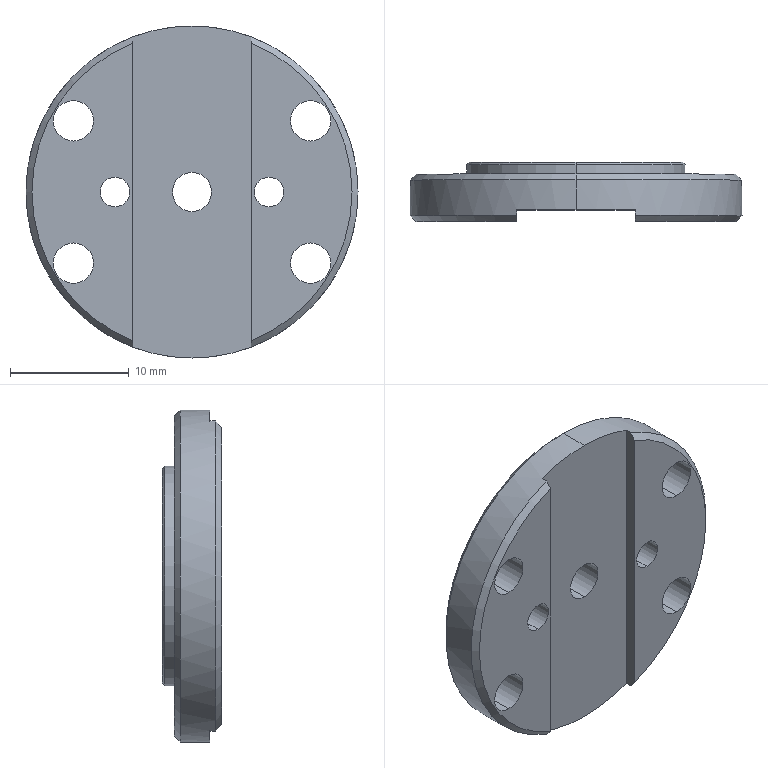Part | SolidWorks | features HoleWzd 3, Chamfer 2, ICE 2, Revolution 1 | 1 solid | 31 faces | box 28 x 5 x 28 mm | volume 2209 mm3 | cylinder 18 | plane 7 | cone 6 | commonest cylinder face diameters 3.4 x8 2.5 x4 3.3 x2 18.5 x2 28 x2
STEP:
#1=CARTESIAN_POINT('',(0.,5.,9.05));
#2=VERTEX_POINT('',#1);
#3=CARTESIAN_POINT('',(0.,5.,-9.05));
#4=VERTEX_POINT('',#3);
#5=CARTESIAN_POINT('',(0.,5.,0.));
#6=DIRECTION('',(0.,1.,0.));
#7=DIRECTION('',(0.,0.,-1.));
#8=AXIS2_PLACEMENT_3D('',#5,#6,#7);
#9=CIRCLE('',#8,9.05);
#10=EDGE_CURVE('',#2,#4,#9,.T.);
#11=ORIENTED_EDGE('',*,*,#10,.F.);
#12=CARTESIAN_POINT('',(0.,4.8,9.25));
#13=VERTEX_POINT('',#12);
#14=CARTESIAN_POINT('',(0.,5.,9.05));
#15=DIRECTION('',(0.,-0.7071,0.7071));
#16=VECTOR('',#15,1000.);
#17=LINE('',#14,#16);
#18=EDGE_CURVE('',#2,#13,#17,.T.);
#19=ORIENTED_EDGE('',*,*,#18,.T.);
#20=CARTESIAN_POINT('',(0.,4.8,-9.25));
#21=VERTEX_POINT('',#20);
#22=CARTESIAN_POINT('',(0.,4.8,0.));
#23=DIRECTION('',(0.,-1.,0.));
#24=DIRECTION('',(0.,0.,-1.));
#25=AXIS2_PLACEMENT_3D('',#22,#23,#24);
#26=CIRCLE('',#25,9.25);
#27=EDGE_CURVE('',#21,#13,#26,.T.);
#28=ORIENTED_EDGE('',*,*,#27,.F.);
#29=CARTESIAN_POINT('',(0.,5.,-9.05));
#30=DIRECTION('',(0.,-0.7071,-0.7071));
#31=VECTOR('',#30,1000.);
#32=LINE('',#29,#31);
#33=EDGE_CURVE('',#4,#21,#32,.T.);
#34=ORIENTED_EDGE('',*,*,#33,.F.);
#35=EDGE_LOOP('',(#11,#19,#28,#34));
#36=FACE_OUTER_BOUND('',#35,.T.);
#37=CARTESIAN_POINT('',(0.,5.,0.));
#38=DIRECTION('',(0.,-1.,0.));
#39=DIRECTION('',(0.,0.,-1.));
#40=AXIS2_PLACEMENT_3D('',#37,#38,#39);
#41=CONICAL_SURFACE('',#40,9.05,0.7854);
#42=ADVANCED_FACE('',(#36),#41,.T.);
#43=CARTESIAN_POINT('',(0.,4.,13.5));
#44=VERTEX_POINT('',#43);
#45=CARTESIAN_POINT('',(0.,4.,-13.5));
#46=VERTEX_POINT('',#45);
#47=CARTESIAN_POINT('',(0.,4.,0.));
#48=DIRECTION('',(0.,1.,0.));
#49=DIRECTION('',(0.,0.,1.));
#50=AXIS2_PLACEMENT_3D('',#47,#48,#49);
#51=CIRCLE('',#50,13.5);
#52=EDGE_CURVE('',#44,#46,#51,.T.);
#53=ORIENTED_EDGE('',*,*,#52,.F.);
#54=CARTESIAN_POINT('',(0.,3.5,14.));
#55=VERTEX_POINT('',#54);
#56=CARTESIAN_POINT('',(0.,3.5,14.));
#57=DIRECTION('',(0.,-0.7071,0.7071));
#58=VECTOR('',#57,1000.);
#59=LINE('',#56,#58);
#60=EDGE_CURVE('',#44,#55,#59,.T.);
#61=ORIENTED_EDGE('',*,*,#60,.T.);
#62=CARTESIAN_POINT('',(0.,3.5,-14.));
#63=VERTEX_POINT('',#62);
#64=CARTESIAN_POINT('',(0.,3.5,0.));
#65=DIRECTION('',(0.,-1.,0.));
#66=DIRECTION('',(0.,0.,1.));
#67=AXIS2_PLACEMENT_3D('',#64,#65,#66);
#68=CIRCLE('',#67,14.);
#69=EDGE_CURVE('',#63,#55,#68,.T.);
#70=ORIENTED_EDGE('',*,*,#69,.F.);
#71=CARTESIAN_POINT('',(0.,3.5,-14.));
#72=DIRECTION('',(0.,-0.7071,-0.7071));
#73=VECTOR('',#72,1000.);
#74=LINE('',#71,#73);
#75=EDGE_CURVE('',#46,#63,#74,.T.);
#76=ORIENTED_EDGE('',*,*,#75,.F.);
#77=EDGE_LOOP('',(#53,#61,#70,#76));
#78=FACE_OUTER_BOUND('',#77,.T.);
#79=CARTESIAN_POINT('',(0.,3.5,0.));
#80=DIRECTION('',(0.,-1.,0.));
#81=DIRECTION('',(0.,0.,-1.));
#82=AXIS2_PLACEMENT_3D('',#79,#80,#81);
#83=CONICAL_SURFACE('',#82,14.,0.7854);
#84=ADVANCED_FACE('',(#78),#83,.T.);
#85=CARTESIAN_POINT('',(0.,5.,1.65));
#86=VERTEX_POINT('',#85);
#87=CARTESIAN_POINT('',(0.,5.,-1.65));
#88=VERTEX_POINT('',#87);
#89=CARTESIAN_POINT('',(0.,5.,0.));
#90=DIRECTION('',(0.,-1.,0.));
#91=DIRECTION('',(0.,0.,-1.));
#92=AXIS2_PLACEMENT_3D('',#89,#90,#91);
#93=CIRCLE('',#92,1.65);
#94=EDGE_CURVE('',#86,#88,#93,.T.);
#95=ORIENTED_EDGE('',*,*,#94,.F.);
#96=CARTESIAN_POINT('',(0.,1.,1.65));
#97=VERTEX_POINT('',#96);
#98=CARTESIAN_POINT('',(0.,1.,1.65));
#99=DIRECTION('',(0.,-1.,0.));
#100=VECTOR('',#99,1000.);
#101=LINE('',#98,#100);
#102=EDGE_CURVE('',#86,#97,#101,.T.);
#103=ORIENTED_EDGE('',*,*,#102,.T.);
#104=CARTESIAN_POINT('',(0.,1.,-1.65));
#105=VERTEX_POINT('',#104);
#106=CARTESIAN_POINT('',(0.,1.,0.));
#107=DIRECTION('',(0.,-1.,0.));
#108=DIRECTION('',(0.,0.,-1.));
#109=AXIS2_PLACEMENT_3D('',#106,#107,#108);
#110=CIRCLE('',#109,1.65);
#111=EDGE_CURVE('',#97,#105,#110,.T.);
#112=ORIENTED_EDGE('',*,*,#111,.T.);
#113=CARTESIAN_POINT('',(0.,1.,-1.65));
#114=DIRECTION('',(0.,-1.,0.));
#115=VECTOR('',#114,1000.);
#116=LINE('',#113,#115);
#117=EDGE_CURVE('',#88,#105,#116,.T.);
#118=ORIENTED_EDGE('',*,*,#117,.F.);
#119=EDGE_LOOP('',(#95,#103,#112,#118));
#120=FACE_OUTER_BOUND('',#119,.T.);
#121=CARTESIAN_POINT('',(0.,1.,0.));
#122=DIRECTION('',(0.,-1.,0.));
#123=DIRECTION('',(0.,0.,-1.));
#124=AXIS2_PLACEMENT_3D('',#121,#122,#123);
#125=CYLINDRICAL_SURFACE('',#124,1.65);
#126=ADVANCED_FACE('',(#120),#125,.F.);
#127=CARTESIAN_POINT('',(-10.,4.,4.3));
#128=VERTEX_POINT('',#127);
#129=CARTESIAN_POINT('',(-10.,4.,7.7));
#130=VERTEX_POINT('',#129);
#131=CARTESIAN_POINT('',(-10.,4.,6.));
#132=DIRECTION('',(0.,1.,0.));
#133=DIRECTION('',(0.,0.,1.));
#134=AXIS2_PLACEMENT_3D('',#131,#132,#133);
#135=CIRCLE('',#134,1.7);
#136=EDGE_CURVE('',#128,#130,#135,.T.);
#137=ORIENTED_EDGE('',*,*,#136,.T.);
#138=CARTESIAN_POINT('',(-10.,0.,7.7));
#139=VERTEX_POINT('',#138);
#140=CARTESIAN_POINT('',(-10.,0.,7.7));
#141=DIRECTION('',(0.,-1.,0.));
#142=VECTOR('',#141,1000.);
#143=LINE('',#140,#142);
#144=EDGE_CURVE('',#130,#139,#143,.T.);
#145=ORIENTED_EDGE('',*,*,#144,.T.);
#146=CARTESIAN_POINT('',(-10.,0.,4.3));
#147=VERTEX_POINT('',#146);
#148=CARTESIAN_POINT('',(-10.,0.,6.));
#149=DIRECTION('',(0.,-1.,0.));
#150=DIRECTION('',(0.,0.,-1.));
#151=AXIS2_PLACEMENT_3D('',#148,#149,#150);
#152=CIRCLE('',#151,1.7);
#153=EDGE_CURVE('',#139,#147,#152,.T.);
#154=ORIENTED_EDGE('',*,*,#153,.T.);
#155=CARTESIAN_POINT('',(-10.,0.,4.3));
#156=DIRECTION('',(0.,-1.,0.));
#157=VECTOR('',#156,1000.);
#158=LINE('',#155,#157);
#159=EDGE_CURVE('',#128,#147,#158,.T.);
#160=ORIENTED_EDGE('',*,*,#159,.F.);
#161=EDGE_LOOP('',(#137,#145,#154,#160));
#162=FACE_OUTER_BOUND('',#161,.T.);
#163=CARTESIAN_POINT('',(-10.,0.,6.));
#164=DIRECTION('',(0.,-1.,0.));
#165=DIRECTION('',(0.,0.,-1.));
#166=AXIS2_PLACEMENT_3D('',#163,#164,#165);
#167=CYLINDRICAL_SURFACE('',#166,1.7);
#168=ADVANCED_FACE('',(#162),#167,.F.);
#169=CARTESIAN_POINT('',(-10.,4.,-7.7));
#170=VERTEX_POINT('',#169);
#171=CARTESIAN_POINT('',(-10.,4.,-4.3));
#172=VERTEX_POINT('',#171);
#173=CARTESIAN_POINT('',(-10.,4.,-6.));
#174=DIRECTION('',(0.,1.,0.));
#175=DIRECTION('',(0.,0.,1.));
#176=AXIS2_PLACEMENT_3D('',#173,#174,#175);
#177=CIRCLE('',#176,1.7);
#178=EDGE_CURVE('',#170,#172,#177,.T.);
#179=ORIENTED_EDGE('',*,*,#178,.T.);
#180=CARTESIAN_POINT('',(-10.,0.,-4.3));
#181=VERTEX_POINT('',#180);
#182=CARTESIAN_POINT('',(-10.,0.,-4.3));
#183=DIRECTION('',(0.,-1.,0.));
#184=VECTOR('',#183,1000.);
#185=LINE('',#182,#184);
#186=EDGE_CURVE('',#172,#181,#185,.T.);
#187=ORIENTED_EDGE('',*,*,#186,.T.);
#188=CARTESIAN_POINT('',(-10.,0.,-7.7));
#189=VERTEX_POINT('',#188);
#190=CARTESIAN_POINT('',(-10.,0.,-6.));
#191=DIRECTION('',(0.,-1.,0.));
#192=DIRECTION('',(0.,0.,-1.));
#193=AXIS2_PLACEMENT_3D('',#190,#191,#192);
#194=CIRCLE('',#193,1.7);
#195=EDGE_CURVE('',#181,#189,#194,.T.);
#196=ORIENTED_EDGE('',*,*,#195,.T.);
#197=CARTESIAN_POINT('',(-10.,0.,-7.7));
#198=DIRECTION('',(0.,-1.,0.));
#199=VECTOR('',#198,1000.);
#200=LINE('',#197,#199);
#201=EDGE_CURVE('',#170,#189,#200,.T.);
#202=ORIENTED_EDGE('',*,*,#201,.F.);
#203=EDGE_LOOP('',(#179,#187,#196,#202));
#204=FACE_OUTER_BOUND('',#203,.T.);
#205=CARTESIAN_POINT('',(-10.,0.,-6.));
#206=DIRECTION('',(0.,-1.,0.));
#207=DIRECTION('',(0.,0.,-1.));
#208=AXIS2_PLACEMENT_3D('',#205,#206,#207);
#209=CYLINDRICAL_SURFACE('',#208,1.7);
#210=ADVANCED_FACE('',(#204),#209,.F.);
#211=CARTESIAN_POINT('',(10.,4.,4.3));
#212=VERTEX_POINT('',#211);
#213=CARTESIAN_POINT('',(10.,4.,7.7));
#214=VERTEX_POINT('',#213);
#215=CARTESIAN_POINT('',(10.,4.,6.));
#216=DIRECTION('',(0.,1.,0.));
#217=DIRECTION('',(0.,0.,1.));
#218=AXIS2_PLACEMENT_3D('',#215,#216,#217);
#219=CIRCLE('',#218,1.7);
#220=EDGE_CURVE('',#212,#214,#219,.T.);
#221=ORIENTED_EDGE('',*,*,#220,.T.);
#222=CARTESIAN_POINT('',(10.,0.,7.7));
#223=VERTEX_POINT('',#222);
#224=CARTESIAN_POINT('',(10.,0.,7.7));
#225=DIRECTION('',(0.,-1.,0.));
#226=VECTOR('',#225,1000.);
#227=LINE('',#224,#226);
#228=EDGE_CURVE('',#214,#223,#227,.T.);
#229=ORIENTED_EDGE('',*,*,#228,.T.);
#230=CARTESIAN_POINT('',(10.,0.,4.3));
#231=VERTEX_POINT('',#230);
#232=CARTESIAN_POINT('',(10.,0.,6.));
#233=DIRECTION('',(0.,-1.,0.));
#234=DIRECTION('',(0.,0.,-1.));
#235=AXIS2_PLACEMENT_3D('',#232,#233,#234);
#236=CIRCLE('',#235,1.7);
#237=EDGE_CURVE('',#223,#231,#236,.T.);
#238=ORIENTED_EDGE('',*,*,#237,.T.);
#239=CARTESIAN_POINT('',(10.,0.,4.3));
#240=DIRECTION('',(0.,-1.,0.));
#241=VECTOR('',#240,1000.);
#242=LINE('',#239,#241);
#243=EDGE_CURVE('',#212,#231,#242,.T.);
#244=ORIENTED_EDGE('',*,*,#243,.F.);
#245=EDGE_LOOP('',(#221,#229,#238,#244));
#246=FACE_OUTER_BOUND('',#245,.T.);
#247=CARTESIAN_POINT('',(10.,0.,6.));
#248=DIRECTION('',(0.,-1.,0.));
#249=DIRECTION('',(0.,0.,-1.));
#250=AXIS2_PLACEMENT_3D('',#247,#248,#249);
#251=CYLINDRICAL_SURFACE('',#250,1.7);
#252=ADVANCED_FACE('',(#246),#251,.F.);
#253=CARTESIAN_POINT('',(10.,4.,-7.7));
#254=VERTEX_POINT('',#253);
#255=CARTESIAN_POINT('',(10.,4.,-4.3));
#256=VERTEX_POINT('',#255);
#257=CARTESIAN_POINT('',(10.,4.,-6.));
#258=DIRECTION('',(0.,1.,0.));
#259=DIRECTION('',(0.,0.,1.));
#260=AXIS2_PLACEMENT_3D('',#257,#258,#259);
#261=CIRCLE('',#260,1.7);
#262=EDGE_CURVE('',#254,#256,#261,.T.);
#263=ORIENTED_EDGE('',*,*,#262,.T.);
#264=CARTESIAN_POINT('',(10.,0.,-4.3));
#265=VERTEX_POINT('',#264);
#266=CARTESIAN_POINT('',(10.,0.,-4.3));
#267=DIRECTION('',(0.,-1.,0.));
#268=VECTOR('',#267,1000.);
#269=LINE('',#266,#268);
#270=EDGE_CURVE('',#256,#265,#269,.T.);
#271=ORIENTED_EDGE('',*,*,#270,.T.);
#272=CARTESIAN_POINT('',(10.,0.,-7.7));
#273=VERTEX_POINT('',#272);
#274=CARTESIAN_POINT('',(10.,0.,-6.));
#275=DIRECTION('',(0.,-1.,0.));
#276=DIRECTION('',(0.,0.,-1.));
#277=AXIS2_PLACEMENT_3D('',#274,#275,#276);
#278=CIRCLE('',#277,1.7);
#279=EDGE_CURVE('',#265,#273,#278,.T.);
#280=ORIENTED_EDGE('',*,*,#279,.T.);
#281=CARTESIAN_POINT('',(10.,0.,-7.7));
#282=DIRECTION('',(0.,-1.,0.));
#283=VECTOR('',#282,1000.);
#284=LINE('',#281,#283);
#285=EDGE_CURVE('',#254,#273,#284,.T.);
#286=ORIENTED_EDGE('',*,*,#285,.F.);
#287=EDGE_LOOP('',(#263,#271,#280,#286));
#288=FACE_OUTER_BOUND('',#287,.T.);
#289=CARTESIAN_POINT('',(10.,0.,-6.));
#290=DIRECTION('',(0.,-1.,0.));
#291=DIRECTION('',(0.,0.,-1.));
#292=AXIS2_PLACEMENT_3D('',#289,#290,#291);
#293=CYLINDRICAL_SURFACE('',#292,1.7);
#294=ADVANCED_FACE('',(#288),#293,.F.);
#295=CARTESIAN_POINT('',(0.,4.,9.25));
#296=VERTEX_POINT('',#295);
#297=CARTESIAN_POINT('',(0.,4.,-9.25));
#298=VERTEX_POINT('',#297);
#299=CARTESIAN_POINT('',(0.,4.,0.));
#300=DIRECTION('',(0.,1.,0.));
#301=DIRECTION('',(0.,0.,1.));
#302=AXIS2_PLACEMENT_3D('',#299,#300,#301);
#303=CIRCLE('',#302,9.25);
#304=EDGE_CURVE('',#296,#298,#303,.T.);
#305=ORIENTED_EDGE('',*,*,#304,.T.);
#306=CARTESIAN_POINT('',(0.,4.,-9.25));
#307=DIRECTION('',(0.,1.,0.));
#308=VECTOR('',#307,1000.);
#309=LINE('',#306,#308);
#310=EDGE_CURVE('',#298,#21,#309,.T.);
#311=ORIENTED_EDGE('',*,*,#310,.T.);
#312=ORIENTED_EDGE('',*,*,#27,.T.);
#313=CARTESIAN_POINT('',(0.,4.,9.25));
#314=DIRECTION('',(0.,1.,0.));
#315=VECTOR('',#314,1000.);
#316=LINE('',#313,#315);
#317=EDGE_CURVE('',#296,#13,#316,.T.);
#318=ORIENTED_EDGE('',*,*,#317,.F.);
#319=EDGE_LOOP('',(#305,#311,#312,#318));
#320=FACE_OUTER_BOUND('',#319,.T.);
#321=CARTESIAN_POINT('',(0.,4.,0.));
#322=DIRECTION('',(0.,1.,0.));
#323=DIRECTION('',(0.,0.,1.));
#324=AXIS2_PLACEMENT_3D('',#321,#322,#323);
#325=CYLINDRICAL_SURFACE('',#324,9.25);
#326=ADVANCED_FACE('',(#320),#325,.T.);
#327=CARTESIAN_POINT('',(-6.5,0.,-1.25));
#328=VERTEX_POINT('',#327);
#329=CARTESIAN_POINT('',(-6.5,0.,1.25));
#330=VERTEX_POINT('',#329);
#331=CARTESIAN_POINT('',(-6.5,0.,0.));
#332=DIRECTION('',(0.,1.,0.));
#333=DIRECTION('',(0.,0.,1.));
#334=AXIS2_PLACEMENT_3D('',#331,#332,#333);
#335=CIRCLE('',#334,1.25);
#336=EDGE_CURVE('',#328,#330,#335,.T.);
#337=ORIENTED_EDGE('',*,*,#336,.F.);
#338=CARTESIAN_POINT('',(-6.5,5.,-1.25));
#339=VERTEX_POINT('',#338);
#340=CARTESIAN_POINT('',(-6.5,5.,-1.25));
#341=DIRECTION('',(0.,1.,0.));
#342=VECTOR('',#341,1000.);
#343=LINE('',#340,#342);
#344=EDGE_CURVE('',#328,#339,#343,.T.);
#345=ORIENTED_EDGE('',*,*,#344,.T.);
#346=CARTESIAN_POINT('',(-6.5,5.,1.25));
#347=VERTEX_POINT('',#346);
#348=CARTESIAN_POINT('',(-6.5,5.,0.));
#349=DIRECTION('',(0.,1.,0.));
#350=DIRECTION('',(0.,0.,1.));
#351=AXIS2_PLACEMENT_3D('',#348,#349,#350);
#352=CIRCLE('',#351,1.25);
#353=EDGE_CURVE('',#339,#347,#352,.T.);
#354=ORIENTED_EDGE('',*,*,#353,.T.);
#355=CARTESIAN_POINT('',(-6.5,5.,1.25));
#356=DIRECTION('',(0.,1.,0.));
#357=VECTOR('',#356,1000.);
#358=LINE('',#355,#357);
#359=EDGE_CURVE('',#330,#347,#358,.T.);
#360=ORIENTED_EDGE('',*,*,#359,.F.);
#361=EDGE_LOOP('',(#337,#345,#354,#360));
#362=FACE_OUTER_BOUND('',#361,.T.);
#363=CARTESIAN_POINT('',(-6.5,5.,0.));
#364=DIRECTION('',(0.,1.,0.));
#365=DIRECTION('',(0.,0.,1.));
#366=AXIS2_PLACEMENT_3D('',#363,#364,#365);
#367=CYLINDRICAL_SURFACE('',#366,1.25);
#368=ADVANCED_FACE('',(#362),#367,.F.);
#369=CARTESIAN_POINT('',(6.5,0.,-1.25));
#370=VERTEX_POINT('',#369);
#371=CARTESIAN_POINT('',(6.5,0.,1.25));
#372=VERTEX_POINT('',#371);
#373=CARTESIAN_POINT('',(6.5,0.,0.));
#374=DIRECTION('',(0.,1.,0.));
#375=DIRECTION('',(0.,0.,1.));
#376=AXIS2_PLACEMENT_3D('',#373,#374,#375);
#377=CIRCLE('',#376,1.25);
#378=EDGE_CURVE('',#370,#372,#377,.T.);
#379=ORIENTED_EDGE('',*,*,#378,.F.);
#380=CARTESIAN_POINT('',(6.5,5.,-1.25));
#381=VERTEX_POINT('',#380);
#382=CARTESIAN_POINT('',(6.5,5.,-1.25));
#383=DIRECTION('',(0.,1.,0.));
#384=VECTOR('',#383,1000.);
#385=LINE('',#382,#384);
#386=EDGE_CURVE('',#370,#381,#385,.T.);
#387=ORIENTED_EDGE('',*,*,#386,.T.);
#388=CARTESIAN_POINT('',(6.5,5.,1.25));
#389=VERTEX_POINT('',#388);
#390=CARTESIAN_POINT('',(6.5,5.,0.));
#391=DIRECTION('',(0.,1.,0.));
#392=DIRECTION('',(0.,0.,1.));
#393=AXIS2_PLACEMENT_3D('',#390,#391,#392);
#394=CIRCLE('',#393,1.25);
#395=EDGE_CURVE('',#381,#389,#394,.T.);
#396=ORIENTED_EDGE('',*,*,#395,.T.);
#397=CARTESIAN_POINT('',(6.5,5.,1.25));
#398=DIRECTION('',(0.,1.,0.));
#399=VECTOR('',#398,1000.);
#400=LINE('',#397,#399);
#401=EDGE_CURVE('',#372,#389,#400,.T.);
#402=ORIENTED_EDGE('',*,*,#401,.F.);
#403=EDGE_LOOP('',(#379,#387,#396,#402));
#404=FACE_OUTER_BOUND('',#403,.T.);
#405=CARTESIAN_POINT('',(6.5,5.,0.));
#406=DIRECTION('',(0.,1.,0.));
#407=DIRECTION('',(0.,0.,1.));
#408=AXIS2_PLACEMENT_3D('',#405,#406,#407);
#409=CYLINDRICAL_SURFACE('',#408,1.25);
#410=ADVANCED_FACE('',(#404),#409,.F.);
#411=ORIENTED_EDGE('',*,*,#69,.T.);
#412=CARTESIAN_POINT('',(0.,1.,14.));
#413=VERTEX_POINT('',#412);
#414=CARTESIAN_POINT('',(0.,0.,14.));
#415=DIRECTION('',(0.,-1.,0.));
#416=VECTOR('',#415,1000.);
#417=LINE('',#414,#416);
#418=EDGE_CURVE('',#55,#413,#417,.T.);
#419=ORIENTED_EDGE('',*,*,#418,.T.);
#420=CARTESIAN_POINT('',(5.,1.,13.077));
#421=VERTEX_POINT('',#420);
#422=CARTESIAN_POINT('',(0.,1.,0.));
#423=DIRECTION('',(0.,-1.,0.));
#424=DIRECTION('',(0.,0.,1.));
#425=AXIS2_PLACEMENT_3D('',#422,#423,#424);
#426=CIRCLE('',#425,14.);
#427=EDGE_CURVE('',#421,#413,#426,.T.);
#428=ORIENTED_EDGE('',*,*,#427,.F.);
#429=CARTESIAN_POINT('',(5.,0.5,13.077));
#430=VERTEX_POINT('',#429);
#431=CARTESIAN_POINT('',(5.,0.,13.077));
#432=DIRECTION('',(0.,1.,0.));
#433=VECTOR('',#432,1000.);
#434=LINE('',#431,#433);
#435=EDGE_CURVE('',#430,#421,#434,.T.);
#436=ORIENTED_EDGE('',*,*,#435,.F.);
#437=CARTESIAN_POINT('',(5.,0.5,-13.077));
#438=VERTEX_POINT('',#437);
#439=CARTESIAN_POINT('',(0.,0.5,0.));
#440=DIRECTION('',(0.,1.,0.));
#441=DIRECTION('',(0.,0.,-1.));
#442=AXIS2_PLACEMENT_3D('',#439,#440,#441);
#443=CIRCLE('',#442,14.);
#444=EDGE_CURVE('',#430,#438,#443,.T.);
#445=ORIENTED_EDGE('',*,*,#444,.T.);
#446=CARTESIAN_POINT('',(5.,1.,-13.077));
#447=VERTEX_POINT('',#446);
#448=CARTESIAN_POINT('',(5.,0.,-13.077));
#449=DIRECTION('',(0.,-1.,0.));
#450=VECTOR('',#449,1000.);
#451=LINE('',#448,#450);
#452=EDGE_CURVE('',#447,#438,#451,.T.);
#453=ORIENTED_EDGE('',*,*,#452,.F.);
#454=CARTESIAN_POINT('',(0.,1.,-14.));
#455=VERTEX_POINT('',#454);
#456=CARTESIAN_POINT('',(0.,1.,0.));
#457=DIRECTION('',(0.,-1.,0.));
#458=DIRECTION('',(0.,0.,1.));
#459=AXIS2_PLACEMENT_3D('',#456,#457,#458);
#460=CIRCLE('',#459,14.);
#461=EDGE_CURVE('',#455,#447,#460,.T.);
#462=ORIENTED_EDGE('',*,*,#461,.F.);
#463=CARTESIAN_POINT('',(0.,0.,-14.));
#464=DIRECTION('',(0.,-1.,0.));
#465=VECTOR('',#464,1000.);
#466=LINE('',#463,#465);
#467=EDGE_CURVE('',#63,#455,#466,.T.);
#468=ORIENTED_EDGE('',*,*,#467,.F.);
#469=EDGE_LOOP('',(#411,#419,#428,#436,#445,#453,#462,#468));
#470=FACE_OUTER_BOUND('',#469,.T.);
#471=CARTESIAN_POINT('',(0.,0.,0.));
#472=DIRECTION('',(0.,-1.,0.));
#473=DIRECTION('',(0.,0.,-1.));
#474=AXIS2_PLACEMENT_3D('',#471,#472,#473);
#475=CYLINDRICAL_SURFACE('',#474,14.);
#476=ADVANCED_FACE('',(#470),#475,.T.);
#477=CARTESIAN_POINT('',(-5.,0.,12.54));
#478=VERTEX_POINT('',#477);
#479=CARTESIAN_POINT('',(-5.,0.,-12.54));
#480=VERTEX_POINT('',#479);
#481=CARTESIAN_POINT('',(-5.,0.,0.));
#482=DIRECTION('',(0.,0.,-1.));
#483=VECTOR('',#482,1000.);
#484=LINE('',#481,#483);
#485=EDGE_CURVE('',#478,#480,#484,.T.);
#486=ORIENTED_EDGE('',*,*,#485,.F.);
#487=CARTESIAN_POINT('',(0.,0.,0.));
#488=DIRECTION('',(0.,-1.,0.));
#489=DIRECTION('',(0.,0.,-1.));
#490=AXIS2_PLACEMENT_3D('',#487,#488,#489);
#491=CIRCLE('',#490,13.5);
#492=EDGE_CURVE('',#478,#480,#491,.T.);
#493=ORIENTED_EDGE('',*,*,#492,.T.);
#494=EDGE_LOOP('',(#486,#493));
#495=FACE_OUTER_BOUND('',#494,.T.);
#496=CARTESIAN_POINT('',(-6.5,0.,0.));
#497=DIRECTION('',(0.,1.,0.));
#498=DIRECTION('',(0.,0.,1.));
#499=AXIS2_PLACEMENT_3D('',#496,#497,#498);
#500=CIRCLE('',#499,1.25);
#501=EDGE_CURVE('',#330,#328,#500,.T.);
#502=ORIENTED_EDGE('',*,*,#501,.T.);
#503=ORIENTED_EDGE('',*,*,#336,.T.);
#504=EDGE_LOOP('',(#502,#503));
#505=FACE_BOUND('',#504,.T.);
#506=CARTESIAN_POINT('',(-10.,0.,-6.));
#507=DIRECTION('',(0.,-1.,0.));
#508=DIRECTION('',(0.,0.,-1.));
#509=AXIS2_PLACEMENT_3D('',#506,#507,#508);
#510=CIRCLE('',#509,1.7);
#511=EDGE_CURVE('',#189,#181,#510,.T.);
#512=ORIENTED_EDGE('',*,*,#511,.F.);
#513=ORIENTED_EDGE('',*,*,#195,.F.);
#514=EDGE_LOOP('',(#512,#513));
#515=FACE_BOUND('',#514,.T.);
#516=CARTESIAN_POINT('',(-10.,0.,6.));
#517=DIRECTION('',(0.,-1.,0.));
#518=DIRECTION('',(0.,0.,-1.));
#519=AXIS2_PLACEMENT_3D('',#516,#517,#518);
#520=CIRCLE('',#519,1.7);
#521=EDGE_CURVE('',#147,#139,#520,.T.);
#522=ORIENTED_EDGE('',*,*,#521,.F.);
#523=ORIENTED_EDGE('',*,*,#153,.F.);
#524=EDGE_LOOP('',(#522,#523));
#525=FACE_BOUND('',#524,.T.);
#526=CARTESIAN_POINT('',(0.,0.,0.));
#527=DIRECTION('',(0.,-1.,0.));
#528=DIRECTION('',(0.,0.,-1.));
#529=AXIS2_PLACEMENT_3D('',#526,#527,#528);
#530=PLANE('',#529);
#531=ADVANCED_FACE('',(#495,#505,#515,#525),#530,.T.);
#532=CARTESIAN_POINT('',(0.,5.,0.));
#533=DIRECTION('',(0.,1.,0.));
#534=DIRECTION('',(0.,0.,-1.));
#535=AXIS2_PLACEMENT_3D('',#532,#533,#534);
#536=CIRCLE('',#535,9.05);
#537=EDGE_CURVE('',#4,#2,#536,.T.);
#538=ORIENTED_EDGE('',*,*,#537,.T.);
#539=ORIENTED_EDGE('',*,*,#10,.T.);
#540=EDGE_LOOP('',(#538,#539));
#541=FACE_OUTER_BOUND('',#540,.T.);
#542=CARTESIAN_POINT('',(0.,5.,0.));
#543=DIRECTION('',(0.,-1.,0.));
#544=DIRECTION('',(0.,0.,-1.));
#545=AXIS2_PLACEMENT_3D('',#542,#543,#544);
#546=CIRCLE('',#545,1.65);
#547=EDGE_CURVE('',#88,#86,#546,.T.);
#548=ORIENTED_EDGE('',*,*,#547,.T.);
#549=ORIENTED_EDGE('',*,*,#94,.T.);
#550=EDGE_LOOP('',(#548,#549));
#551=FACE_BOUND('',#550,.T.);
#552=CARTESIAN_POINT('',(6.5,5.,0.));
#553=DIRECTION('',(0.,1.,0.));
#554=DIRECTION('',(0.,0.,1.));
#555=AXIS2_PLACEMENT_3D('',#552,#553,#554);
#556=CIRCLE('',#555,1.25);
#557=EDGE_CURVE('',#389,#381,#556,.T.);
#558=ORIENTED_EDGE('',*,*,#557,.F.);
#559=ORIENTED_EDGE('',*,*,#395,.F.);
#560=EDGE_LOOP('',(#558,#559));
#561=FACE_BOUND('',#560,.T.);
#562=CARTESIAN_POINT('',(-6.5,5.,0.));
#563=DIRECTION('',(0.,1.,0.));
#564=DIRECTION('',(0.,0.,1.));
#565=AXIS2_PLACEMENT_3D('',#562,#563,#564);
#566=CIRCLE('',#565,1.25);
#567=EDGE_CURVE('',#347,#339,#566,.T.);
#568=ORIENTED_EDGE('',*,*,#567,.F.);
#569=ORIENTED_EDGE('',*,*,#353,.F.);
#570=EDGE_LOOP('',(#568,#569));
#571=FACE_BOUND('',#570,.T.);
#572=CARTESIAN_POINT('',(0.,5.,0.));
#573=DIRECTION('',(0.,-1.,0.));
#574=DIRECTION('',(0.,0.,-1.));
#575=AXIS2_PLACEMENT_3D('',#572,#573,#574);
#576=PLANE('',#575);
#577=ADVANCED_FACE('',(#541,#551,#561,#571),#576,.F.);
#578=ORIENTED_EDGE('',*,*,#418,.F.);
#579=CARTESIAN_POINT('',(0.,3.5,0.));
#580=DIRECTION('',(0.,-1.,0.));
#581=DIRECTION('',(0.,0.,1.));
#582=AXIS2_PLACEMENT_3D('',#579,#580,#581);
#583=CIRCLE('',#582,14.);
#584=EDGE_CURVE('',#55,#63,#583,.T.);
#585=ORIENTED_EDGE('',*,*,#584,.T.);
#586=ORIENTED_EDGE('',*,*,#467,.T.);
#587=CARTESIAN_POINT('',(-5.,1.,-13.077));
#588=VERTEX_POINT('',#587);
#589=CARTESIAN_POINT('',(0.,1.,0.));
#590=DIRECTION('',(0.,-1.,0.));
#591=DIRECTION('',(0.,0.,1.));
#592=AXIS2_PLACEMENT_3D('',#589,#590,#591);
#593=CIRCLE('',#592,14.);
#594=EDGE_CURVE('',#588,#455,#593,.T.);
#595=ORIENTED_EDGE('',*,*,#594,.F.);
#596=CARTESIAN_POINT('',(-5.,0.5,-13.077));
#597=VERTEX_POINT('',#596);
#598=CARTESIAN_POINT('',(-5.,0.,-13.077));
#599=DIRECTION('',(0.,1.,0.));
#600=VECTOR('',#599,1000.);
#601=LINE('',#598,#600);
#602=EDGE_CURVE('',#597,#588,#601,.T.);
#603=ORIENTED_EDGE('',*,*,#602,.F.);
#604=CARTESIAN_POINT('',(-5.,0.5,13.077));
#605=VERTEX_POINT('',#604);
#606=CARTESIAN_POINT('',(0.,0.5,0.));
#607=DIRECTION('',(0.,1.,0.));
#608=DIRECTION('',(0.,0.,-1.));
#609=AXIS2_PLACEMENT_3D('',#606,#607,#608);
#610=CIRCLE('',#609,14.);
#611=EDGE_CURVE('',#597,#605,#610,.T.);
#612=ORIENTED_EDGE('',*,*,#611,.T.);
#613=CARTESIAN_POINT('',(-5.,1.,13.077));
#614=VERTEX_POINT('',#613);
#615=CARTESIAN_POINT('',(-5.,0.,13.077));
#616=DIRECTION('',(0.,-1.,0.));
#617=VECTOR('',#616,1000.);
#618=LINE('',#615,#617);
#619=EDGE_CURVE('',#614,#605,#618,.T.);
#620=ORIENTED_EDGE('',*,*,#619,.F.);
#621=CARTESIAN_POINT('',(0.,1.,0.));
#622=DIRECTION('',(0.,-1.,0.));
#623=DIRECTION('',(0.,0.,1.));
#624=AXIS2_PLACEMENT_3D('',#621,#622,#623);
#625=CIRCLE('',#624,14.);
#626=EDGE_CURVE('',#413,#614,#625,.T.);
#627=ORIENTED_EDGE('',*,*,#626,.F.);
#628=EDGE_LOOP('',(#578,#585,#586,#595,#603,#612,#620,#627));
#629=FACE_OUTER_BOUND('',#628,.T.);
#630=CARTESIAN_POINT('',(0.,0.,0.));
#631=DIRECTION('',(0.,-1.,0.));
#632=DIRECTION('',(0.,0.,-1.));
#633=AXIS2_PLACEMENT_3D('',#630,#631,#632);
#634=CYLINDRICAL_SURFACE('',#633,14.);
#635=ADVANCED_FACE('',(#629),#634,.T.);
#636=CARTESIAN_POINT('',(5.,0.,-12.54));
#637=VERTEX_POINT('',#636);
#638=CARTESIAN_POINT('',(5.,0.,12.54));
#639=VERTEX_POINT('',#638);
#640=CARTESIAN_POINT('',(5.,0.,0.));
#641=DIRECTION('',(0.,0.,1.));
#642=VECTOR('',#641,1000.);
#643=LINE('',#640,#642);
#644=EDGE_CURVE('',#637,#639,#643,.T.);
#645=ORIENTED_EDGE('',*,*,#644,.F.);
#646=CARTESIAN_POINT('',(0.,0.,0.));
#647=DIRECTION('',(0.,-1.,0.));
#648=DIRECTION('',(0.,0.,-1.));
#649=AXIS2_PLACEMENT_3D('',#646,#647,#648);
#650=CIRCLE('',#649,13.5);
#651=EDGE_CURVE('',#637,#639,#650,.T.);
#652=ORIENTED_EDGE('',*,*,#651,.T.);
#653=EDGE_LOOP('',(#645,#652));
#654=FACE_OUTER_BOUND('',#653,.T.);
#655=CARTESIAN_POINT('',(10.,0.,6.));
#656=DIRECTION('',(0.,-1.,0.));
#657=DIRECTION('',(0.,0.,-1.));
#658=AXIS2_PLACEMENT_3D('',#655,#656,#657);
#659=CIRCLE('',#658,1.7);
#660=EDGE_CURVE('',#231,#223,#659,.T.);
#661=ORIENTED_EDGE('',*,*,#660,.F.);
#662=ORIENTED_EDGE('',*,*,#237,.F.);
#663=EDGE_LOOP('',(#661,#662));
#664=FACE_BOUND('',#663,.T.);
#665=CARTESIAN_POINT('',(10.,0.,-6.));
#666=DIRECTION('',(0.,-1.,0.));
#667=DIRECTION('',(0.,0.,-1.));
#668=AXIS2_PLACEMENT_3D('',#665,#666,#667);
#669=CIRCLE('',#668,1.7);
#670=EDGE_CURVE('',#273,#265,#669,.T.);
#671=ORIENTED_EDGE('',*,*,#670,.F.);
#672=ORIENTED_EDGE('',*,*,#279,.F.);
#673=EDGE_LOOP('',(#671,#672));
#674=FACE_BOUND('',#673,.T.);
#675=CARTESIAN_POINT('',(6.5,0.,0.));
#676=DIRECTION('',(0.,1.,0.));
#677=DIRECTION('',(0.,0.,1.));
#678=AXIS2_PLACEMENT_3D('',#675,#676,#677);
#679=CIRCLE('',#678,1.25);
#680=EDGE_CURVE('',#372,#370,#679,.T.);
#681=ORIENTED_EDGE('',*,*,#680,.T.);
#682=ORIENTED_EDGE('',*,*,#378,.T.);
#683=EDGE_LOOP('',(#681,#682));
#684=FACE_BOUND('',#683,.T.);
#685=CARTESIAN_POINT('',(0.,0.,0.));
#686=DIRECTION('',(0.,-1.,0.));
#687=DIRECTION('',(0.,0.,-1.));
#688=AXIS2_PLACEMENT_3D('',#685,#686,#687);
#689=PLANE('',#688);
#690=ADVANCED_FACE('',(#654,#664,#674,#684),#689,.T.);
#691=ORIENTED_EDGE('',*,*,#386,.F.);
#692=ORIENTED_EDGE('',*,*,#680,.F.);
#693=ORIENTED_EDGE('',*,*,#401,.T.);
#694=ORIENTED_EDGE('',*,*,#557,.T.);
#695=EDGE_LOOP('',(#691,#692,#693,#694));
#696=FACE_OUTER_BOUND('',#695,.T.);
#697=CARTESIAN_POINT('',(6.5,5.,0.));
#698=DIRECTION('',(0.,1.,0.));
#699=DIRECTION('',(0.,0.,1.));
#700=AXIS2_PLACEMENT_3D('',#697,#698,#699);
#701=CYLINDRICAL_SURFACE('',#700,1.25);
#702=ADVANCED_FACE('',(#696),#701,.F.);
#703=ORIENTED_EDGE('',*,*,#344,.F.);
#704=ORIENTED_EDGE('',*,*,#501,.F.);
#705=ORIENTED_EDGE('',*,*,#359,.T.);
#706=ORIENTED_EDGE('',*,*,#567,.T.);
#707=EDGE_LOOP('',(#703,#704,#705,#706));
#708=FACE_OUTER_BOUND('',#707,.T.);
#709=CARTESIAN_POINT('',(-6.5,5.,0.));
#710=DIRECTION('',(0.,1.,0.));
#711=DIRECTION('',(0.,0.,1.));
#712=AXIS2_PLACEMENT_3D('',#709,#710,#711);
#713=CYLINDRICAL_SURFACE('',#712,1.25);
#714=ADVANCED_FACE('',(#708),#713,.F.);
#715=CARTESIAN_POINT('',(0.,4.,0.));
#716=DIRECTION('',(0.,1.,0.));
#717=DIRECTION('',(0.,0.,1.));
#718=AXIS2_PLACEMENT_3D('',#715,#716,#717);
#719=CIRCLE('',#718,13.5);
#720=EDGE_CURVE('',#46,#44,#719,.T.);
#721=ORIENTED_EDGE('',*,*,#720,.T.);
#722=ORIENTED_EDGE('',*,*,#52,.T.);
#723=EDGE_LOOP('',(#721,#722));
#724=FACE_OUTER_BOUND('',#723,.T.);
#725=ORIENTED_EDGE('',*,*,#136,.F.);
#726=CARTESIAN_POINT('',(-10.,4.,6.));
#727=DIRECTION('',(0.,1.,0.));
#728=DIRECTION('',(0.,0.,1.));
#729=AXIS2_PLACEMENT_3D('',#726,#727,#728);
#730=CIRCLE('',#729,1.7);
#731=EDGE_CURVE('',#130,#128,#730,.T.);
#732=ORIENTED_EDGE('',*,*,#731,.F.);
#733=EDGE_LOOP('',(#725,#732));
#734=FACE_BOUND('',#733,.T.);
#735=ORIENTED_EDGE('',*,*,#178,.F.);
#736=CARTESIAN_POINT('',(-10.,4.,-6.));
#737=DIRECTION('',(0.,1.,0.));
#738=DIRECTION('',(0.,0.,1.));
#739=AXIS2_PLACEMENT_3D('',#736,#737,#738);
#740=CIRCLE('',#739,1.7);
#741=EDGE_CURVE('',#172,#170,#740,.T.);
#742=ORIENTED_EDGE('',*,*,#741,.F.);
#743=EDGE_LOOP('',(#735,#742));
#744=FACE_BOUND('',#743,.T.);
#745=ORIENTED_EDGE('',*,*,#220,.F.);
#746=CARTESIAN_POINT('',(10.,4.,6.));
#747=DIRECTION('',(0.,1.,0.));
#748=DIRECTION('',(0.,0.,1.));
#749=AXIS2_PLACEMENT_3D('',#746,#747,#748);
#750=CIRCLE('',#749,1.7);
#751=EDGE_CURVE('',#214,#212,#750,.T.);
#752=ORIENTED_EDGE('',*,*,#751,.F.);
#753=EDGE_LOOP('',(#745,#752));
#754=FACE_BOUND('',#753,.T.);
#755=ORIENTED_EDGE('',*,*,#262,.F.);
#756=CARTESIAN_POINT('',(10.,4.,-6.));
#757=DIRECTION('',(0.,1.,0.));
#758=DIRECTION('',(0.,0.,1.));
#759=AXIS2_PLACEMENT_3D('',#756,#757,#758);
#760=CIRCLE('',#759,1.7);
#761=EDGE_CURVE('',#256,#254,#760,.T.);
#762=ORIENTED_EDGE('',*,*,#761,.F.);
#763=EDGE_LOOP('',(#755,#762));
#764=FACE_BOUND('',#763,.T.);
#765=ORIENTED_EDGE('',*,*,#304,.F.);
#766=CARTESIAN_POINT('',(0.,4.,0.));
#767=DIRECTION('',(0.,1.,0.));
#768=DIRECTION('',(0.,0.,1.));
#769=AXIS2_PLACEMENT_3D('',#766,#767,#768);
#770=CIRCLE('',#769,9.25);
#771=EDGE_CURVE('',#298,#296,#770,.T.);
#772=ORIENTED_EDGE('',*,*,#771,.F.);
#773=EDGE_LOOP('',(#765,#772));
#774=FACE_BOUND('',#773,.T.);
#775=CARTESIAN_POINT('',(0.,4.,0.));
#776=DIRECTION('',(0.,1.,0.));
#777=DIRECTION('',(0.,0.,1.));
#778=AXIS2_PLACEMENT_3D('',#775,#776,#777);
#779=PLANE('',#778);
#780=ADVANCED_FACE('',(#724,#734,#744,#754,#764,#774),#779,.T.);
#781=ORIENTED_EDGE('',*,*,#310,.F.);
#782=ORIENTED_EDGE('',*,*,#771,.T.);
#783=ORIENTED_EDGE('',*,*,#317,.T.);
#784=CARTESIAN_POINT('',(0.,4.8,0.));
#785=DIRECTION('',(0.,-1.,0.));
#786=DIRECTION('',(0.,0.,-1.));
#787=AXIS2_PLACEMENT_3D('',#784,#785,#786);
#788=CIRCLE('',#787,9.25);
#789=EDGE_CURVE('',#13,#21,#788,.T.);
#790=ORIENTED_EDGE('',*,*,#789,.T.);
#791=EDGE_LOOP('',(#781,#782,#783,#790));
#792=FACE_OUTER_BOUND('',#791,.T.);
#793=CARTESIAN_POINT('',(0.,4.,0.));
#794=DIRECTION('',(0.,1.,0.));
#795=DIRECTION('',(0.,0.,1.));
#796=AXIS2_PLACEMENT_3D('',#793,#794,#795);
#797=CYLINDRICAL_SURFACE('',#796,9.25);
#798=ADVANCED_FACE('',(#792),#797,.T.);
#799=ORIENTED_EDGE('',*,*,#270,.F.);
#800=ORIENTED_EDGE('',*,*,#761,.T.);
#801=ORIENTED_EDGE('',*,*,#285,.T.);
#802=ORIENTED_EDGE('',*,*,#670,.T.);
#803=EDGE_LOOP('',(#799,#800,#801,#802));
#804=FACE_OUTER_BOUND('',#803,.T.);
#805=CARTESIAN_POINT('',(10.,0.,-6.));
#806=DIRECTION('',(0.,-1.,0.));
#807=DIRECTION('',(0.,0.,-1.));
#808=AXIS2_PLACEMENT_3D('',#805,#806,#807);
#809=CYLINDRICAL_SURFACE('',#808,1.7);
#810=ADVANCED_FACE('',(#804),#809,.F.);
#811=ORIENTED_EDGE('',*,*,#228,.F.);
#812=ORIENTED_EDGE('',*,*,#751,.T.);
#813=ORIENTED_EDGE('',*,*,#243,.T.);
#814=ORIENTED_EDGE('',*,*,#660,.T.);
#815=EDGE_LOOP('',(#811,#812,#813,#814));
#816=FACE_OUTER_BOUND('',#815,.T.);
#817=CARTESIAN_POINT('',(10.,0.,6.));
#818=DIRECTION('',(0.,-1.,0.));
#819=DIRECTION('',(0.,0.,-1.));
#820=AXIS2_PLACEMENT_3D('',#817,#818,#819);
#821=CYLINDRICAL_SURFACE('',#820,1.7);
#822=ADVANCED_FACE('',(#816),#821,.F.);
#823=ORIENTED_EDGE('',*,*,#186,.F.);
#824=ORIENTED_EDGE('',*,*,#741,.T.);
#825=ORIENTED_EDGE('',*,*,#201,.T.);
#826=ORIENTED_EDGE('',*,*,#511,.T.);
#827=EDGE_LOOP('',(#823,#824,#825,#826));
#828=FACE_OUTER_BOUND('',#827,.T.);
#829=CARTESIAN_POINT('',(-10.,0.,-6.));
#830=DIRECTION('',(0.,-1.,0.));
#831=DIRECTION('',(0.,0.,-1.));
#832=AXIS2_PLACEMENT_3D('',#829,#830,#831);
#833=CYLINDRICAL_SURFACE('',#832,1.7);
#834=ADVANCED_FACE('',(#828),#833,.F.);
#835=ORIENTED_EDGE('',*,*,#144,.F.);
#836=ORIENTED_EDGE('',*,*,#731,.T.);
#837=ORIENTED_EDGE('',*,*,#159,.T.);
#838=ORIENTED_EDGE('',*,*,#521,.T.);
#839=EDGE_LOOP('',(#835,#836,#837,#838));
#840=FACE_OUTER_BOUND('',#839,.T.);
#841=CARTESIAN_POINT('',(-10.,0.,6.));
#842=DIRECTION('',(0.,-1.,0.));
#843=DIRECTION('',(0.,0.,-1.));
#844=AXIS2_PLACEMENT_3D('',#841,#842,#843);
#845=CYLINDRICAL_SURFACE('',#844,1.7);
#846=ADVANCED_FACE('',(#840),#845,.F.);
#847=ORIENTED_EDGE('',*,*,#485,.T.);
#848=CARTESIAN_POINT('',(-5.,0.,-12.54));
#849=CARTESIAN_POINT('',(-5.,0.1664,-12.719));
#850=CARTESIAN_POINT('',(-5.,0.3331,-12.898));
#851=CARTESIAN_POINT('',(-5.,0.5,-13.077));
#852=B_SPLINE_CURVE_WITH_KNOTS('',3,(#848,#849,#850,#851),.UNSPECIFIED.,.F.,.F.,(4,4),(0.,0.0007336),.UNSPECIFIED.);
#853=EDGE_CURVE('',#480,#597,#852,.T.);
#854=ORIENTED_EDGE('',*,*,#853,.T.);
#855=ORIENTED_EDGE('',*,*,#602,.T.);
#856=CARTESIAN_POINT('',(-5.,1.,15.714));
#857=DIRECTION('',(0.,0.,-1.));
#858=VECTOR('',#857,1000.);
#859=LINE('',#856,#858);
#860=EDGE_CURVE('',#614,#588,#859,.T.);
#861=ORIENTED_EDGE('',*,*,#860,.F.);
#862=ORIENTED_EDGE('',*,*,#619,.T.);
#863=CARTESIAN_POINT('',(-5.,0.5,13.077));
#864=CARTESIAN_POINT('',(-5.,0.3331,12.898));
#865=CARTESIAN_POINT('',(-5.,0.1664,12.719));
#866=CARTESIAN_POINT('',(-5.,0.,12.54));
#867=B_SPLINE_CURVE_WITH_KNOTS('',3,(#863,#864,#865,#866),.UNSPECIFIED.,.F.,.F.,(4,4),(0.,0.0007336),.UNSPECIFIED.);
#868=EDGE_CURVE('',#605,#478,#867,.T.);
#869=ORIENTED_EDGE('',*,*,#868,.T.);
#870=EDGE_LOOP('',(#847,#854,#855,#861,#862,#869));
#871=FACE_OUTER_BOUND('',#870,.T.);
#872=CARTESIAN_POINT('',(-5.,1.,15.714));
#873=DIRECTION('',(-1.,0.,0.));
#874=DIRECTION('',(0.,0.,1.));
#875=AXIS2_PLACEMENT_3D('',#872,#873,#874);
#876=PLANE('',#875);
#877=ADVANCED_FACE('',(#871),#876,.F.);
#878=ORIENTED_EDGE('',*,*,#644,.T.);
#879=CARTESIAN_POINT('',(5.,0.,12.54));
#880=CARTESIAN_POINT('',(5.,0.1664,12.719));
#881=CARTESIAN_POINT('',(5.,0.3331,12.898));
#882=CARTESIAN_POINT('',(5.,0.5,13.077));
#883=B_SPLINE_CURVE_WITH_KNOTS('',3,(#879,#880,#881,#882),.UNSPECIFIED.,.F.,.F.,(4,4),(0.,0.0007336),.UNSPECIFIED.);
#884=EDGE_CURVE('',#639,#430,#883,.T.);
#885=ORIENTED_EDGE('',*,*,#884,.T.);
#886=ORIENTED_EDGE('',*,*,#435,.T.);
#887=CARTESIAN_POINT('',(5.,1.,15.714));
#888=DIRECTION('',(0.,0.,1.));
#889=VECTOR('',#888,1000.);
#890=LINE('',#887,#889);
#891=EDGE_CURVE('',#447,#421,#890,.T.);
#892=ORIENTED_EDGE('',*,*,#891,.F.);
#893=ORIENTED_EDGE('',*,*,#452,.T.);
#894=CARTESIAN_POINT('',(5.,0.5,-13.077));
#895=CARTESIAN_POINT('',(5.,0.3331,-12.898));
#896=CARTESIAN_POINT('',(5.,0.1664,-12.719));
#897=CARTESIAN_POINT('',(5.,0.,-12.54));
#898=B_SPLINE_CURVE_WITH_KNOTS('',3,(#894,#895,#896,#897),.UNSPECIFIED.,.F.,.F.,(4,4),(0.,0.0007336),.UNSPECIFIED.);
#899=EDGE_CURVE('',#438,#637,#898,.T.);
#900=ORIENTED_EDGE('',*,*,#899,.T.);
#901=EDGE_LOOP('',(#878,#885,#886,#892,#893,#900));
#902=FACE_OUTER_BOUND('',#901,.T.);
#903=CARTESIAN_POINT('',(5.,1.,15.714));
#904=DIRECTION('',(1.,0.,0.));
#905=DIRECTION('',(0.,0.,-1.));
#906=AXIS2_PLACEMENT_3D('',#903,#904,#905);
#907=PLANE('',#906);
#908=ADVANCED_FACE('',(#902),#907,.F.);
#909=CARTESIAN_POINT('',(0.,1.,0.));
#910=DIRECTION('',(0.,-1.,0.));
#911=DIRECTION('',(0.,0.,-1.));
#912=AXIS2_PLACEMENT_3D('',#909,#910,#911);
#913=CIRCLE('',#912,1.65);
#914=EDGE_CURVE('',#105,#97,#913,.T.);
#915=ORIENTED_EDGE('',*,*,#914,.F.);
#916=ORIENTED_EDGE('',*,*,#111,.F.);
#917=EDGE_LOOP('',(#915,#916));
#918=FACE_BOUND('',#917,.T.);
#919=ORIENTED_EDGE('',*,*,#594,.T.);
#920=ORIENTED_EDGE('',*,*,#461,.T.);
#921=ORIENTED_EDGE('',*,*,#891,.T.);
#922=ORIENTED_EDGE('',*,*,#427,.T.);
#923=ORIENTED_EDGE('',*,*,#626,.T.);
#924=ORIENTED_EDGE('',*,*,#860,.T.);
#925=EDGE_LOOP('',(#919,#920,#921,#922,#923,#924));
#926=FACE_OUTER_BOUND('',#925,.T.);
#927=CARTESIAN_POINT('',(0.,1.,0.));
#928=DIRECTION('',(0.,1.,0.));
#929=DIRECTION('',(0.,0.,1.));
#930=AXIS2_PLACEMENT_3D('',#927,#928,#929);
#931=PLANE('',#930);
#932=ADVANCED_FACE('',(#918,#926),#931,.F.);
#933=ORIENTED_EDGE('',*,*,#102,.F.);
#934=ORIENTED_EDGE('',*,*,#547,.F.);
#935=ORIENTED_EDGE('',*,*,#117,.T.);
#936=ORIENTED_EDGE('',*,*,#914,.T.);
#937=EDGE_LOOP('',(#933,#934,#935,#936));
#938=FACE_OUTER_BOUND('',#937,.T.);
#939=CARTESIAN_POINT('',(0.,1.,0.));
#940=DIRECTION('',(0.,-1.,0.));
#941=DIRECTION('',(0.,0.,-1.));
#942=AXIS2_PLACEMENT_3D('',#939,#940,#941);
#943=CYLINDRICAL_SURFACE('',#942,1.65);
#944=ADVANCED_FACE('',(#938),#943,.F.);
#945=ORIENTED_EDGE('',*,*,#60,.F.);
#946=ORIENTED_EDGE('',*,*,#720,.F.);
#947=ORIENTED_EDGE('',*,*,#75,.T.);
#948=ORIENTED_EDGE('',*,*,#584,.F.);
#949=EDGE_LOOP('',(#945,#946,#947,#948));
#950=FACE_OUTER_BOUND('',#949,.T.);
#951=CARTESIAN_POINT('',(0.,3.5,0.));
#952=DIRECTION('',(0.,-1.,0.));
#953=DIRECTION('',(0.,0.,-1.));
#954=AXIS2_PLACEMENT_3D('',#951,#952,#953);
#955=CONICAL_SURFACE('',#954,14.,0.7854);
#956=ADVANCED_FACE('',(#950),#955,.T.);
#957=ORIENTED_EDGE('',*,*,#899,.F.);
#958=ORIENTED_EDGE('',*,*,#444,.F.);
#959=ORIENTED_EDGE('',*,*,#884,.F.);
#960=ORIENTED_EDGE('',*,*,#651,.F.);
#961=EDGE_LOOP('',(#957,#958,#959,#960));
#962=FACE_OUTER_BOUND('',#961,.T.);
#963=CARTESIAN_POINT('',(0.,0.,0.));
#964=DIRECTION('',(0.,1.,0.));
#965=DIRECTION('',(0.,0.,1.));
#966=AXIS2_PLACEMENT_3D('',#963,#964,#965);
#967=CONICAL_SURFACE('',#966,13.5,0.7854);
#968=ADVANCED_FACE('',(#962),#967,.T.);
#969=ORIENTED_EDGE('',*,*,#868,.F.);
#970=ORIENTED_EDGE('',*,*,#611,.F.);
#971=ORIENTED_EDGE('',*,*,#853,.F.);
#972=ORIENTED_EDGE('',*,*,#492,.F.);
#973=EDGE_LOOP('',(#969,#970,#971,#972));
#974=FACE_OUTER_BOUND('',#973,.T.);
#975=CARTESIAN_POINT('',(0.,0.,0.));
#976=DIRECTION('',(0.,1.,0.));
#977=DIRECTION('',(0.,0.,1.));
#978=AXIS2_PLACEMENT_3D('',#975,#976,#977);
#979=CONICAL_SURFACE('',#978,13.5,0.7854);
#980=ADVANCED_FACE('',(#974),#979,.T.);
#981=ORIENTED_EDGE('',*,*,#18,.F.);
#982=ORIENTED_EDGE('',*,*,#537,.F.);
#983=ORIENTED_EDGE('',*,*,#33,.T.);
#984=ORIENTED_EDGE('',*,*,#789,.F.);
#985=EDGE_LOOP('',(#981,#982,#983,#984));
#986=FACE_OUTER_BOUND('',#985,.T.);
#987=CARTESIAN_POINT('',(0.,5.,0.));
#988=DIRECTION('',(0.,-1.,0.));
#989=DIRECTION('',(0.,0.,-1.));
#990=AXIS2_PLACEMENT_3D('',#987,#988,#989);
#991=CONICAL_SURFACE('',#990,9.05,0.7854);
#992=ADVANCED_FACE('',(#986),#991,.T.);
#993=CLOSED_SHELL('',(#42,#84,#126,#168,#210,#252,#294,#326,#368,#410,#476,#531,#577,#635,#690,#702,#714,#780,#798,#810,#822,#834,#846,#877,#908,#932,#944,#956,#968,#980,#992));
#994=MANIFOLD_SOLID_BREP('',#993);
#995=CARTESIAN_POINT('',(0.,0.,0.));
#996=DIRECTION('',(0.,0.,1.));
#997=DIRECTION('',(1.,0.,0.));
#998=AXIS2_PLACEMENT_3D('',#995,#996,#997);
#999=(LENGTH_UNIT()NAMED_UNIT(*)SI_UNIT(.MILLI.,.METRE.));
#1000=UNCERTAINTY_MEASURE_WITH_UNIT(LENGTH_MEASURE(0.00001),#999,'','');
#1001=(NAMED_UNIT(*)PLANE_ANGLE_UNIT()SI_UNIT($,.RADIAN.));
#1002=(NAMED_UNIT(*)SI_UNIT($,.STERADIAN.)SOLID_ANGLE_UNIT());
#1003=(GEOMETRIC_REPRESENTATION_CONTEXT(3)GLOBAL_UNCERTAINTY_ASSIGNED_CONTEXT((#1000))GLOBAL_UNIT_ASSIGNED_CONTEXT((#999,#1001,#1002))REPRESENTATION_CONTEXT('',''));
#1004=ADVANCED_BREP_SHAPE_REPRESENTATION('',(#994,#998),#1003);